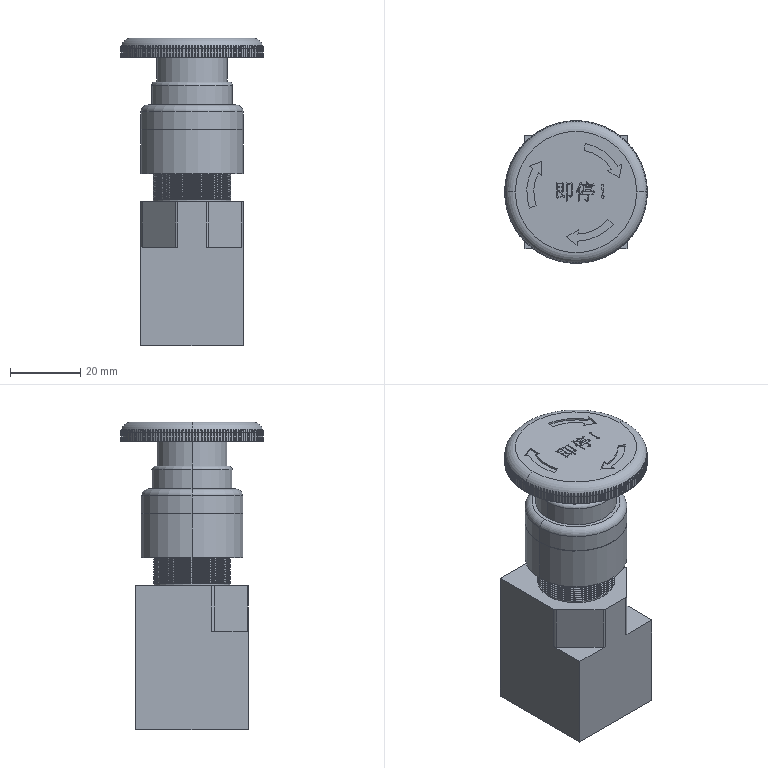Part | SolidWorks | features ICE 10, Fillet 4, CirPattern 2, RevCut 2, Extrusion 1, LPattern 1 | 1 solid | 814 faces | box 40.499 x 40.499 x 87.5 mm | volume 63476 mm3 | plane 548 | cylinder 180 | torus 54 | spline 32 | commonest cylinder face diameters 40.5 x140 22 x22 2 x4 29 x4 24 x3 28 x3